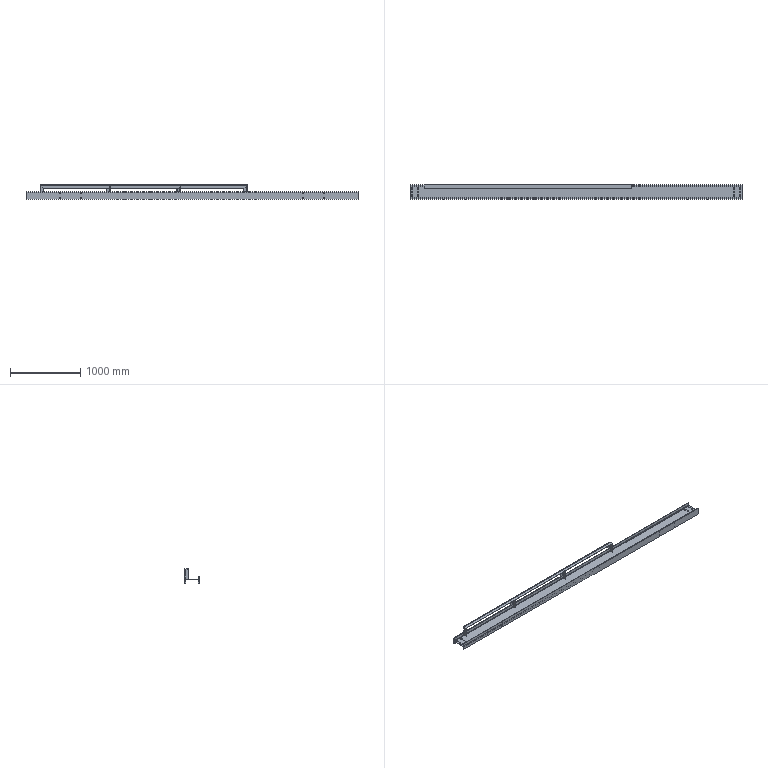Part | STEP file | 休息台主梁2主体_Default<As Machined> | 6 solids | 125 faces | box 4730 x 200 x 200 mm | volume 13901578 mm3 | plane 66 | cylinder 59 | commonest cylinder face diameters 19 x24 15 x16 2.66 x10 11 x5 16 x4